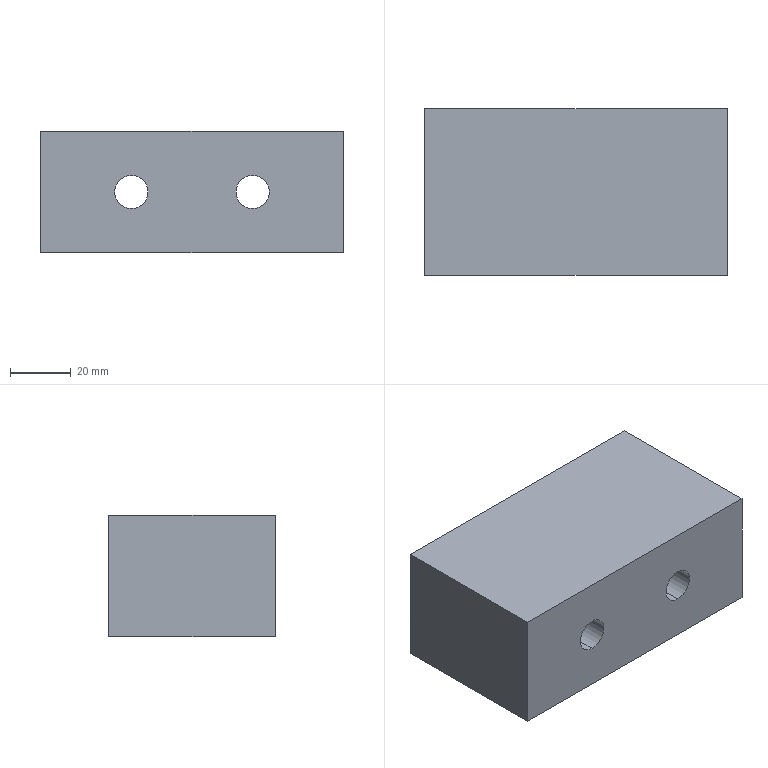Part | SolidWorks | features Extrusion 1, ICE 1 | 1 solid | 16 faces | box 100 x 55 x 40 mm | volume 203169 mm3 | cylinder 8 | plane 8 | commonest cylinder face diameters 11 x4 18 x4
STEP:
#1=CARTESIAN_POINT('',(-20.,35.,-9.));
#2=VERTEX_POINT('',#1);
#3=CARTESIAN_POINT('',(-20.,35.,9.));
#4=VERTEX_POINT('',#3);
#5=CARTESIAN_POINT('',(-20.,35.,0.));
#6=DIRECTION('',(0.,1.,0.));
#7=DIRECTION('',(0.,0.,1.));
#8=AXIS2_PLACEMENT_3D('',#5,#6,#7);
#9=CIRCLE('',#8,9.);
#10=EDGE_CURVE('',#2,#4,#9,.T.);
#11=ORIENTED_EDGE('',*,*,#10,.F.);
#12=CARTESIAN_POINT('',(-20.,55.,-9.));
#13=VERTEX_POINT('',#12);
#14=CARTESIAN_POINT('',(-20.,35.,-9.));
#15=DIRECTION('',(0.,1.,0.));
#16=VECTOR('',#15,1000.);
#17=LINE('',#14,#16);
#18=EDGE_CURVE('',#2,#13,#17,.T.);
#19=ORIENTED_EDGE('',*,*,#18,.T.);
#20=CARTESIAN_POINT('',(-20.,55.,9.));
#21=VERTEX_POINT('',#20);
#22=CARTESIAN_POINT('',(-20.,55.,0.));
#23=DIRECTION('',(0.,1.,0.));
#24=DIRECTION('',(0.,0.,1.));
#25=AXIS2_PLACEMENT_3D('',#22,#23,#24);
#26=CIRCLE('',#25,9.);
#27=EDGE_CURVE('',#13,#21,#26,.T.);
#28=ORIENTED_EDGE('',*,*,#27,.T.);
#29=CARTESIAN_POINT('',(-20.,35.,9.));
#30=DIRECTION('',(0.,1.,0.));
#31=VECTOR('',#30,1000.);
#32=LINE('',#29,#31);
#33=EDGE_CURVE('',#4,#21,#32,.T.);
#34=ORIENTED_EDGE('',*,*,#33,.F.);
#35=EDGE_LOOP('',(#11,#19,#28,#34));
#36=FACE_OUTER_BOUND('',#35,.T.);
#37=CARTESIAN_POINT('',(-20.,35.,0.));
#38=DIRECTION('',(0.,1.,0.));
#39=DIRECTION('',(0.,0.,1.));
#40=AXIS2_PLACEMENT_3D('',#37,#38,#39);
#41=CYLINDRICAL_SURFACE('',#40,9.);
#42=ADVANCED_FACE('',(#36),#41,.F.);
#43=CARTESIAN_POINT('',(20.,35.,-9.));
#44=VERTEX_POINT('',#43);
#45=CARTESIAN_POINT('',(20.,35.,9.));
#46=VERTEX_POINT('',#45);
#47=CARTESIAN_POINT('',(20.,35.,0.));
#48=DIRECTION('',(0.,1.,0.));
#49=DIRECTION('',(0.,0.,1.));
#50=AXIS2_PLACEMENT_3D('',#47,#48,#49);
#51=CIRCLE('',#50,9.);
#52=EDGE_CURVE('',#44,#46,#51,.T.);
#53=ORIENTED_EDGE('',*,*,#52,.F.);
#54=CARTESIAN_POINT('',(20.,55.,-9.));
#55=VERTEX_POINT('',#54);
#56=CARTESIAN_POINT('',(20.,35.,-9.));
#57=DIRECTION('',(0.,1.,0.));
#58=VECTOR('',#57,1000.);
#59=LINE('',#56,#58);
#60=EDGE_CURVE('',#44,#55,#59,.T.);
#61=ORIENTED_EDGE('',*,*,#60,.T.);
#62=CARTESIAN_POINT('',(20.,55.,9.));
#63=VERTEX_POINT('',#62);
#64=CARTESIAN_POINT('',(20.,55.,0.));
#65=DIRECTION('',(0.,1.,0.));
#66=DIRECTION('',(0.,0.,1.));
#67=AXIS2_PLACEMENT_3D('',#64,#65,#66);
#68=CIRCLE('',#67,9.);
#69=EDGE_CURVE('',#55,#63,#68,.T.);
#70=ORIENTED_EDGE('',*,*,#69,.T.);
#71=CARTESIAN_POINT('',(20.,35.,9.));
#72=DIRECTION('',(0.,1.,0.));
#73=VECTOR('',#72,1000.);
#74=LINE('',#71,#73);
#75=EDGE_CURVE('',#46,#63,#74,.T.);
#76=ORIENTED_EDGE('',*,*,#75,.F.);
#77=EDGE_LOOP('',(#53,#61,#70,#76));
#78=FACE_OUTER_BOUND('',#77,.T.);
#79=CARTESIAN_POINT('',(20.,35.,0.));
#80=DIRECTION('',(0.,1.,0.));
#81=DIRECTION('',(0.,0.,1.));
#82=AXIS2_PLACEMENT_3D('',#79,#80,#81);
#83=CYLINDRICAL_SURFACE('',#82,9.);
#84=ADVANCED_FACE('',(#78),#83,.F.);
#85=CARTESIAN_POINT('',(20.,35.,-5.5));
#86=VERTEX_POINT('',#85);
#87=CARTESIAN_POINT('',(20.,35.,5.5));
#88=VERTEX_POINT('',#87);
#89=CARTESIAN_POINT('',(20.,35.,0.));
#90=DIRECTION('',(0.,1.,0.));
#91=DIRECTION('',(0.,0.,1.));
#92=AXIS2_PLACEMENT_3D('',#89,#90,#91);
#93=CIRCLE('',#92,5.5);
#94=EDGE_CURVE('',#86,#88,#93,.T.);
#95=ORIENTED_EDGE('',*,*,#94,.T.);
#96=CARTESIAN_POINT('',(20.,0.,5.5));
#97=VERTEX_POINT('',#96);
#98=CARTESIAN_POINT('',(20.,55.,5.5));
#99=DIRECTION('',(0.,-1.,0.));
#100=VECTOR('',#99,1000.);
#101=LINE('',#98,#100);
#102=EDGE_CURVE('',#88,#97,#101,.T.);
#103=ORIENTED_EDGE('',*,*,#102,.T.);
#104=CARTESIAN_POINT('',(20.,0.,-5.5));
#105=VERTEX_POINT('',#104);
#106=CARTESIAN_POINT('',(20.,0.,0.));
#107=DIRECTION('',(0.,1.,0.));
#108=DIRECTION('',(0.,0.,1.));
#109=AXIS2_PLACEMENT_3D('',#106,#107,#108);
#110=CIRCLE('',#109,5.5);
#111=EDGE_CURVE('',#105,#97,#110,.T.);
#112=ORIENTED_EDGE('',*,*,#111,.F.);
#113=CARTESIAN_POINT('',(20.,55.,-5.5));
#114=DIRECTION('',(0.,-1.,0.));
#115=VECTOR('',#114,1000.);
#116=LINE('',#113,#115);
#117=EDGE_CURVE('',#86,#105,#116,.T.);
#118=ORIENTED_EDGE('',*,*,#117,.F.);
#119=EDGE_LOOP('',(#95,#103,#112,#118));
#120=FACE_OUTER_BOUND('',#119,.T.);
#121=CARTESIAN_POINT('',(20.,55.,0.));
#122=DIRECTION('',(0.,-1.,0.));
#123=DIRECTION('',(0.,0.,-1.));
#124=AXIS2_PLACEMENT_3D('',#121,#122,#123);
#125=CYLINDRICAL_SURFACE('',#124,5.5);
#126=ADVANCED_FACE('',(#120),#125,.F.);
#127=CARTESIAN_POINT('',(-20.,35.,-5.5));
#128=VERTEX_POINT('',#127);
#129=CARTESIAN_POINT('',(-20.,35.,5.5));
#130=VERTEX_POINT('',#129);
#131=CARTESIAN_POINT('',(-20.,35.,0.));
#132=DIRECTION('',(0.,1.,0.));
#133=DIRECTION('',(0.,0.,1.));
#134=AXIS2_PLACEMENT_3D('',#131,#132,#133);
#135=CIRCLE('',#134,5.5);
#136=EDGE_CURVE('',#128,#130,#135,.T.);
#137=ORIENTED_EDGE('',*,*,#136,.T.);
#138=CARTESIAN_POINT('',(-20.,0.,5.5));
#139=VERTEX_POINT('',#138);
#140=CARTESIAN_POINT('',(-20.,55.,5.5));
#141=DIRECTION('',(0.,-1.,0.));
#142=VECTOR('',#141,1000.);
#143=LINE('',#140,#142);
#144=EDGE_CURVE('',#130,#139,#143,.T.);
#145=ORIENTED_EDGE('',*,*,#144,.T.);
#146=CARTESIAN_POINT('',(-20.,0.,-5.5));
#147=VERTEX_POINT('',#146);
#148=CARTESIAN_POINT('',(-20.,0.,0.));
#149=DIRECTION('',(0.,1.,0.));
#150=DIRECTION('',(0.,0.,1.));
#151=AXIS2_PLACEMENT_3D('',#148,#149,#150);
#152=CIRCLE('',#151,5.5);
#153=EDGE_CURVE('',#147,#139,#152,.T.);
#154=ORIENTED_EDGE('',*,*,#153,.F.);
#155=CARTESIAN_POINT('',(-20.,55.,-5.5));
#156=DIRECTION('',(0.,-1.,0.));
#157=VECTOR('',#156,1000.);
#158=LINE('',#155,#157);
#159=EDGE_CURVE('',#128,#147,#158,.T.);
#160=ORIENTED_EDGE('',*,*,#159,.F.);
#161=EDGE_LOOP('',(#137,#145,#154,#160));
#162=FACE_OUTER_BOUND('',#161,.T.);
#163=CARTESIAN_POINT('',(-20.,55.,0.));
#164=DIRECTION('',(0.,-1.,0.));
#165=DIRECTION('',(0.,0.,-1.));
#166=AXIS2_PLACEMENT_3D('',#163,#164,#165);
#167=CYLINDRICAL_SURFACE('',#166,5.5);
#168=ADVANCED_FACE('',(#162),#167,.F.);
#169=ORIENTED_EDGE('',*,*,#144,.F.);
#170=CARTESIAN_POINT('',(-20.,35.,0.));
#171=DIRECTION('',(0.,1.,0.));
#172=DIRECTION('',(0.,0.,1.));
#173=AXIS2_PLACEMENT_3D('',#170,#171,#172);
#174=CIRCLE('',#173,5.5);
#175=EDGE_CURVE('',#130,#128,#174,.T.);
#176=ORIENTED_EDGE('',*,*,#175,.T.);
#177=ORIENTED_EDGE('',*,*,#159,.T.);
#178=CARTESIAN_POINT('',(-20.,0.,0.));
#179=DIRECTION('',(0.,1.,0.));
#180=DIRECTION('',(0.,0.,1.));
#181=AXIS2_PLACEMENT_3D('',#178,#179,#180);
#182=CIRCLE('',#181,5.5);
#183=EDGE_CURVE('',#139,#147,#182,.T.);
#184=ORIENTED_EDGE('',*,*,#183,.F.);
#185=EDGE_LOOP('',(#169,#176,#177,#184));
#186=FACE_OUTER_BOUND('',#185,.T.);
#187=CARTESIAN_POINT('',(-20.,55.,0.));
#188=DIRECTION('',(0.,-1.,0.));
#189=DIRECTION('',(0.,0.,-1.));
#190=AXIS2_PLACEMENT_3D('',#187,#188,#189);
#191=CYLINDRICAL_SURFACE('',#190,5.5);
#192=ADVANCED_FACE('',(#186),#191,.F.);
#193=ORIENTED_EDGE('',*,*,#102,.F.);
#194=CARTESIAN_POINT('',(20.,35.,0.));
#195=DIRECTION('',(0.,1.,0.));
#196=DIRECTION('',(0.,0.,1.));
#197=AXIS2_PLACEMENT_3D('',#194,#195,#196);
#198=CIRCLE('',#197,5.5);
#199=EDGE_CURVE('',#88,#86,#198,.T.);
#200=ORIENTED_EDGE('',*,*,#199,.T.);
#201=ORIENTED_EDGE('',*,*,#117,.T.);
#202=CARTESIAN_POINT('',(20.,0.,0.));
#203=DIRECTION('',(0.,1.,0.));
#204=DIRECTION('',(0.,0.,1.));
#205=AXIS2_PLACEMENT_3D('',#202,#203,#204);
#206=CIRCLE('',#205,5.5);
#207=EDGE_CURVE('',#97,#105,#206,.T.);
#208=ORIENTED_EDGE('',*,*,#207,.F.);
#209=EDGE_LOOP('',(#193,#200,#201,#208));
#210=FACE_OUTER_BOUND('',#209,.T.);
#211=CARTESIAN_POINT('',(20.,55.,0.));
#212=DIRECTION('',(0.,-1.,0.));
#213=DIRECTION('',(0.,0.,-1.));
#214=AXIS2_PLACEMENT_3D('',#211,#212,#213);
#215=CYLINDRICAL_SURFACE('',#214,5.5);
#216=ADVANCED_FACE('',(#210),#215,.F.);
#217=CARTESIAN_POINT('',(20.,55.,0.));
#218=DIRECTION('',(0.,1.,0.));
#219=DIRECTION('',(0.,0.,1.));
#220=AXIS2_PLACEMENT_3D('',#217,#218,#219);
#221=CIRCLE('',#220,9.);
#222=EDGE_CURVE('',#63,#55,#221,.T.);
#223=ORIENTED_EDGE('',*,*,#222,.F.);
#224=ORIENTED_EDGE('',*,*,#69,.F.);
#225=EDGE_LOOP('',(#223,#224));
#226=FACE_BOUND('',#225,.T.);
#227=CARTESIAN_POINT('',(-20.,55.,0.));
#228=DIRECTION('',(0.,1.,0.));
#229=DIRECTION('',(0.,0.,1.));
#230=AXIS2_PLACEMENT_3D('',#227,#228,#229);
#231=CIRCLE('',#230,9.);
#232=EDGE_CURVE('',#21,#13,#231,.T.);
#233=ORIENTED_EDGE('',*,*,#232,.F.);
#234=ORIENTED_EDGE('',*,*,#27,.F.);
#235=EDGE_LOOP('',(#233,#234));
#236=FACE_BOUND('',#235,.T.);
#237=CARTESIAN_POINT('',(50.,55.,20.));
#238=VERTEX_POINT('',#237);
#239=CARTESIAN_POINT('',(50.,55.,-20.));
#240=VERTEX_POINT('',#239);
#241=CARTESIAN_POINT('',(50.,55.,20.));
#242=DIRECTION('',(0.,0.,-1.));
#243=VECTOR('',#242,1000.);
#244=LINE('',#241,#243);
#245=EDGE_CURVE('',#238,#240,#244,.T.);
#246=ORIENTED_EDGE('',*,*,#245,.T.);
#247=CARTESIAN_POINT('',(-50.,55.,-20.));
#248=VERTEX_POINT('',#247);
#249=CARTESIAN_POINT('',(-50.,55.,-20.));
#250=DIRECTION('',(-1.,0.,0.));
#251=VECTOR('',#250,1000.);
#252=LINE('',#249,#251);
#253=EDGE_CURVE('',#240,#248,#252,.T.);
#254=ORIENTED_EDGE('',*,*,#253,.T.);
#255=CARTESIAN_POINT('',(-50.,55.,20.));
#256=VERTEX_POINT('',#255);
#257=CARTESIAN_POINT('',(-50.,55.,20.));
#258=DIRECTION('',(0.,0.,1.));
#259=VECTOR('',#258,1000.);
#260=LINE('',#257,#259);
#261=EDGE_CURVE('',#248,#256,#260,.T.);
#262=ORIENTED_EDGE('',*,*,#261,.T.);
#263=CARTESIAN_POINT('',(-50.,55.,20.));
#264=DIRECTION('',(1.,0.,0.));
#265=VECTOR('',#264,1000.);
#266=LINE('',#263,#265);
#267=EDGE_CURVE('',#256,#238,#266,.T.);
#268=ORIENTED_EDGE('',*,*,#267,.T.);
#269=EDGE_LOOP('',(#246,#254,#262,#268));
#270=FACE_OUTER_BOUND('',#269,.T.);
#271=CARTESIAN_POINT('',(0.,55.,0.));
#272=DIRECTION('',(0.,-1.,0.));
#273=DIRECTION('',(0.,0.,-1.));
#274=AXIS2_PLACEMENT_3D('',#271,#272,#273);
#275=PLANE('',#274);
#276=ADVANCED_FACE('',(#226,#236,#270),#275,.F.);
#277=ORIENTED_EDGE('',*,*,#153,.T.);
#278=ORIENTED_EDGE('',*,*,#183,.T.);
#279=EDGE_LOOP('',(#277,#278));
#280=FACE_BOUND('',#279,.T.);
#281=CARTESIAN_POINT('',(50.,0.,20.));
#282=VERTEX_POINT('',#281);
#283=CARTESIAN_POINT('',(50.,0.,-20.));
#284=VERTEX_POINT('',#283);
#285=CARTESIAN_POINT('',(50.,0.,20.));
#286=DIRECTION('',(0.,0.,-1.));
#287=VECTOR('',#286,1000.);
#288=LINE('',#285,#287);
#289=EDGE_CURVE('',#282,#284,#288,.T.);
#290=ORIENTED_EDGE('',*,*,#289,.F.);
#291=CARTESIAN_POINT('',(-50.,0.,20.));
#292=VERTEX_POINT('',#291);
#293=CARTESIAN_POINT('',(-50.,0.,20.));
#294=DIRECTION('',(1.,0.,0.));
#295=VECTOR('',#294,1000.);
#296=LINE('',#293,#295);
#297=EDGE_CURVE('',#292,#282,#296,.T.);
#298=ORIENTED_EDGE('',*,*,#297,.F.);
#299=CARTESIAN_POINT('',(-50.,0.,-20.));
#300=VERTEX_POINT('',#299);
#301=CARTESIAN_POINT('',(-50.,0.,20.));
#302=DIRECTION('',(0.,0.,1.));
#303=VECTOR('',#302,1000.);
#304=LINE('',#301,#303);
#305=EDGE_CURVE('',#300,#292,#304,.T.);
#306=ORIENTED_EDGE('',*,*,#305,.F.);
#307=CARTESIAN_POINT('',(-50.,0.,-20.));
#308=DIRECTION('',(-1.,0.,0.));
#309=VECTOR('',#308,1000.);
#310=LINE('',#307,#309);
#311=EDGE_CURVE('',#284,#300,#310,.T.);
#312=ORIENTED_EDGE('',*,*,#311,.F.);
#313=EDGE_LOOP('',(#290,#298,#306,#312));
#314=FACE_OUTER_BOUND('',#313,.T.);
#315=ORIENTED_EDGE('',*,*,#111,.T.);
#316=ORIENTED_EDGE('',*,*,#207,.T.);
#317=EDGE_LOOP('',(#315,#316));
#318=FACE_BOUND('',#317,.T.);
#319=CARTESIAN_POINT('',(0.,0.,0.));
#320=DIRECTION('',(0.,-1.,0.));
#321=DIRECTION('',(0.,0.,-1.));
#322=AXIS2_PLACEMENT_3D('',#319,#320,#321);
#323=PLANE('',#322);
#324=ADVANCED_FACE('',(#280,#314,#318),#323,.T.);
#325=ORIENTED_EDGE('',*,*,#289,.T.);
#326=CARTESIAN_POINT('',(50.,55.,-20.));
#327=DIRECTION('',(0.,-1.,0.));
#328=VECTOR('',#327,1000.);
#329=LINE('',#326,#328);
#330=EDGE_CURVE('',#240,#284,#329,.T.);
#331=ORIENTED_EDGE('',*,*,#330,.F.);
#332=ORIENTED_EDGE('',*,*,#245,.F.);
#333=CARTESIAN_POINT('',(50.,55.,20.));
#334=DIRECTION('',(0.,-1.,0.));
#335=VECTOR('',#334,1000.);
#336=LINE('',#333,#335);
#337=EDGE_CURVE('',#238,#282,#336,.T.);
#338=ORIENTED_EDGE('',*,*,#337,.T.);
#339=EDGE_LOOP('',(#325,#331,#332,#338));
#340=FACE_OUTER_BOUND('',#339,.T.);
#341=CARTESIAN_POINT('',(50.,55.,20.));
#342=DIRECTION('',(-1.,0.,0.));
#343=DIRECTION('',(0.,0.,1.));
#344=AXIS2_PLACEMENT_3D('',#341,#342,#343);
#345=PLANE('',#344);
#346=ADVANCED_FACE('',(#340),#345,.F.);
#347=ORIENTED_EDGE('',*,*,#311,.T.);
#348=CARTESIAN_POINT('',(-50.,55.,-20.));
#349=DIRECTION('',(0.,-1.,0.));
#350=VECTOR('',#349,1000.);
#351=LINE('',#348,#350);
#352=EDGE_CURVE('',#248,#300,#351,.T.);
#353=ORIENTED_EDGE('',*,*,#352,.F.);
#354=ORIENTED_EDGE('',*,*,#253,.F.);
#355=ORIENTED_EDGE('',*,*,#330,.T.);
#356=EDGE_LOOP('',(#347,#353,#354,#355));
#357=FACE_OUTER_BOUND('',#356,.T.);
#358=CARTESIAN_POINT('',(-50.,55.,-20.));
#359=DIRECTION('',(0.,0.,1.));
#360=DIRECTION('',(1.,0.,0.));
#361=AXIS2_PLACEMENT_3D('',#358,#359,#360);
#362=PLANE('',#361);
#363=ADVANCED_FACE('',(#357),#362,.F.);
#364=ORIENTED_EDGE('',*,*,#305,.T.);
#365=CARTESIAN_POINT('',(-50.,55.,20.));
#366=DIRECTION('',(0.,-1.,0.));
#367=VECTOR('',#366,1000.);
#368=LINE('',#365,#367);
#369=EDGE_CURVE('',#256,#292,#368,.T.);
#370=ORIENTED_EDGE('',*,*,#369,.F.);
#371=ORIENTED_EDGE('',*,*,#261,.F.);
#372=ORIENTED_EDGE('',*,*,#352,.T.);
#373=EDGE_LOOP('',(#364,#370,#371,#372));
#374=FACE_OUTER_BOUND('',#373,.T.);
#375=CARTESIAN_POINT('',(-50.,55.,20.));
#376=DIRECTION('',(1.,0.,0.));
#377=DIRECTION('',(0.,0.,-1.));
#378=AXIS2_PLACEMENT_3D('',#375,#376,#377);
#379=PLANE('',#378);
#380=ADVANCED_FACE('',(#374),#379,.F.);
#381=ORIENTED_EDGE('',*,*,#297,.T.);
#382=ORIENTED_EDGE('',*,*,#337,.F.);
#383=ORIENTED_EDGE('',*,*,#267,.F.);
#384=ORIENTED_EDGE('',*,*,#369,.T.);
#385=EDGE_LOOP('',(#381,#382,#383,#384));
#386=FACE_OUTER_BOUND('',#385,.T.);
#387=CARTESIAN_POINT('',(-50.,55.,20.));
#388=DIRECTION('',(0.,0.,-1.));
#389=DIRECTION('',(-1.,0.,0.));
#390=AXIS2_PLACEMENT_3D('',#387,#388,#389);
#391=PLANE('',#390);
#392=ADVANCED_FACE('',(#386),#391,.F.);
#393=ORIENTED_EDGE('',*,*,#60,.F.);
#394=CARTESIAN_POINT('',(20.,35.,0.));
#395=DIRECTION('',(0.,1.,0.));
#396=DIRECTION('',(0.,0.,1.));
#397=AXIS2_PLACEMENT_3D('',#394,#395,#396);
#398=CIRCLE('',#397,9.);
#399=EDGE_CURVE('',#46,#44,#398,.T.);
#400=ORIENTED_EDGE('',*,*,#399,.F.);
#401=ORIENTED_EDGE('',*,*,#75,.T.);
#402=ORIENTED_EDGE('',*,*,#222,.T.);
#403=EDGE_LOOP('',(#393,#400,#401,#402));
#404=FACE_OUTER_BOUND('',#403,.T.);
#405=CARTESIAN_POINT('',(20.,35.,0.));
#406=DIRECTION('',(0.,1.,0.));
#407=DIRECTION('',(0.,0.,1.));
#408=AXIS2_PLACEMENT_3D('',#405,#406,#407);
#409=CYLINDRICAL_SURFACE('',#408,9.);
#410=ADVANCED_FACE('',(#404),#409,.F.);
#411=ORIENTED_EDGE('',*,*,#94,.F.);
#412=ORIENTED_EDGE('',*,*,#199,.F.);
#413=EDGE_LOOP('',(#411,#412));
#414=FACE_BOUND('',#413,.T.);
#415=ORIENTED_EDGE('',*,*,#399,.T.);
#416=ORIENTED_EDGE('',*,*,#52,.T.);
#417=EDGE_LOOP('',(#415,#416));
#418=FACE_OUTER_BOUND('',#417,.T.);
#419=CARTESIAN_POINT('',(20.,35.,0.));
#420=DIRECTION('',(0.,1.,0.));
#421=DIRECTION('',(0.,0.,1.));
#422=AXIS2_PLACEMENT_3D('',#419,#420,#421);
#423=PLANE('',#422);
#424=ADVANCED_FACE('',(#414,#418),#423,.T.);
#425=ORIENTED_EDGE('',*,*,#18,.F.);
#426=CARTESIAN_POINT('',(-20.,35.,0.));
#427=DIRECTION('',(0.,1.,0.));
#428=DIRECTION('',(0.,0.,1.));
#429=AXIS2_PLACEMENT_3D('',#426,#427,#428);
#430=CIRCLE('',#429,9.);
#431=EDGE_CURVE('',#4,#2,#430,.T.);
#432=ORIENTED_EDGE('',*,*,#431,.F.);
#433=ORIENTED_EDGE('',*,*,#33,.T.);
#434=ORIENTED_EDGE('',*,*,#232,.T.);
#435=EDGE_LOOP('',(#425,#432,#433,#434));
#436=FACE_OUTER_BOUND('',#435,.T.);
#437=CARTESIAN_POINT('',(-20.,35.,0.));
#438=DIRECTION('',(0.,1.,0.));
#439=DIRECTION('',(0.,0.,1.));
#440=AXIS2_PLACEMENT_3D('',#437,#438,#439);
#441=CYLINDRICAL_SURFACE('',#440,9.);
#442=ADVANCED_FACE('',(#436),#441,.F.);
#443=ORIENTED_EDGE('',*,*,#136,.F.);
#444=ORIENTED_EDGE('',*,*,#175,.F.);
#445=EDGE_LOOP('',(#443,#444));
#446=FACE_BOUND('',#445,.T.);
#447=ORIENTED_EDGE('',*,*,#431,.T.);
#448=ORIENTED_EDGE('',*,*,#10,.T.);
#449=EDGE_LOOP('',(#447,#448));
#450=FACE_OUTER_BOUND('',#449,.T.);
#451=CARTESIAN_POINT('',(-20.,35.,0.));
#452=DIRECTION('',(0.,1.,0.));
#453=DIRECTION('',(0.,0.,1.));
#454=AXIS2_PLACEMENT_3D('',#451,#452,#453);
#455=PLANE('',#454);
#456=ADVANCED_FACE('',(#446,#450),#455,.T.);
#457=CLOSED_SHELL('',(#42,#84,#126,#168,#192,#216,#276,#324,#346,#363,#380,#392,#410,#424,#442,#456));
#458=MANIFOLD_SOLID_BREP('',#457);
#459=CARTESIAN_POINT('',(0.,0.,0.));
#460=DIRECTION('',(0.,0.,1.));
#461=DIRECTION('',(1.,0.,0.));
#462=AXIS2_PLACEMENT_3D('',#459,#460,#461);
#463=(LENGTH_UNIT()NAMED_UNIT(*)SI_UNIT(.MILLI.,.METRE.));
#464=UNCERTAINTY_MEASURE_WITH_UNIT(LENGTH_MEASURE(0.00001),#463,'','');
#465=(NAMED_UNIT(*)PLANE_ANGLE_UNIT()SI_UNIT($,.RADIAN.));
#466=(NAMED_UNIT(*)SI_UNIT($,.STERADIAN.)SOLID_ANGLE_UNIT());
#467=(GEOMETRIC_REPRESENTATION_CONTEXT(3)GLOBAL_UNCERTAINTY_ASSIGNED_CONTEXT((#464))GLOBAL_UNIT_ASSIGNED_CONTEXT((#463,#465,#466))REPRESENTATION_CONTEXT('',''));
#468=ADVANCED_BREP_SHAPE_REPRESENTATION('',(#458,#462),#467);